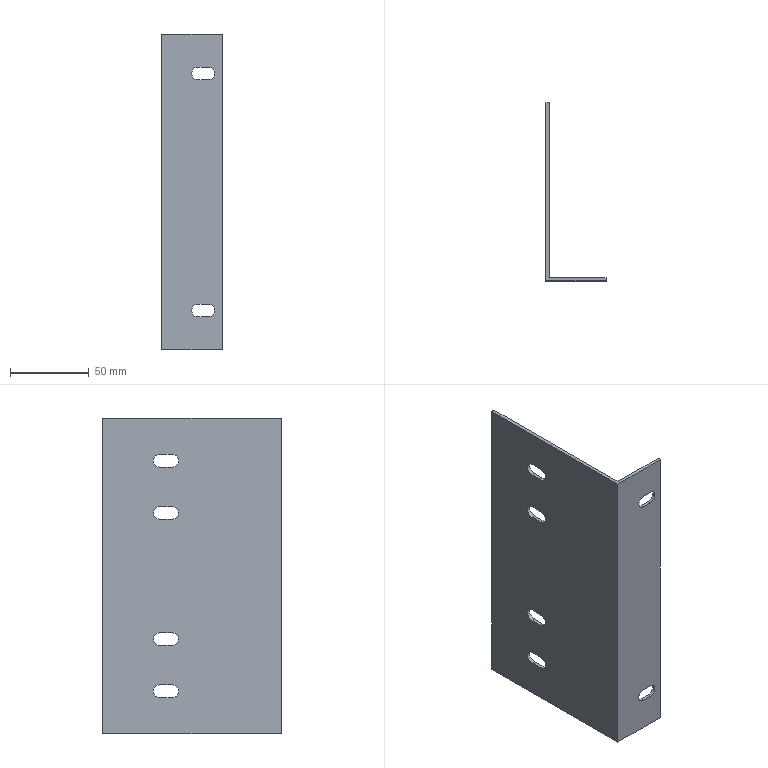Part | STEP file | PN_0027_default | 1 solid | 32 faces | box 38 x 113 x 200 mm | volume 58277 mm3 | plane 20 | cylinder 12 | commonest cylinder face diameters 8 x12